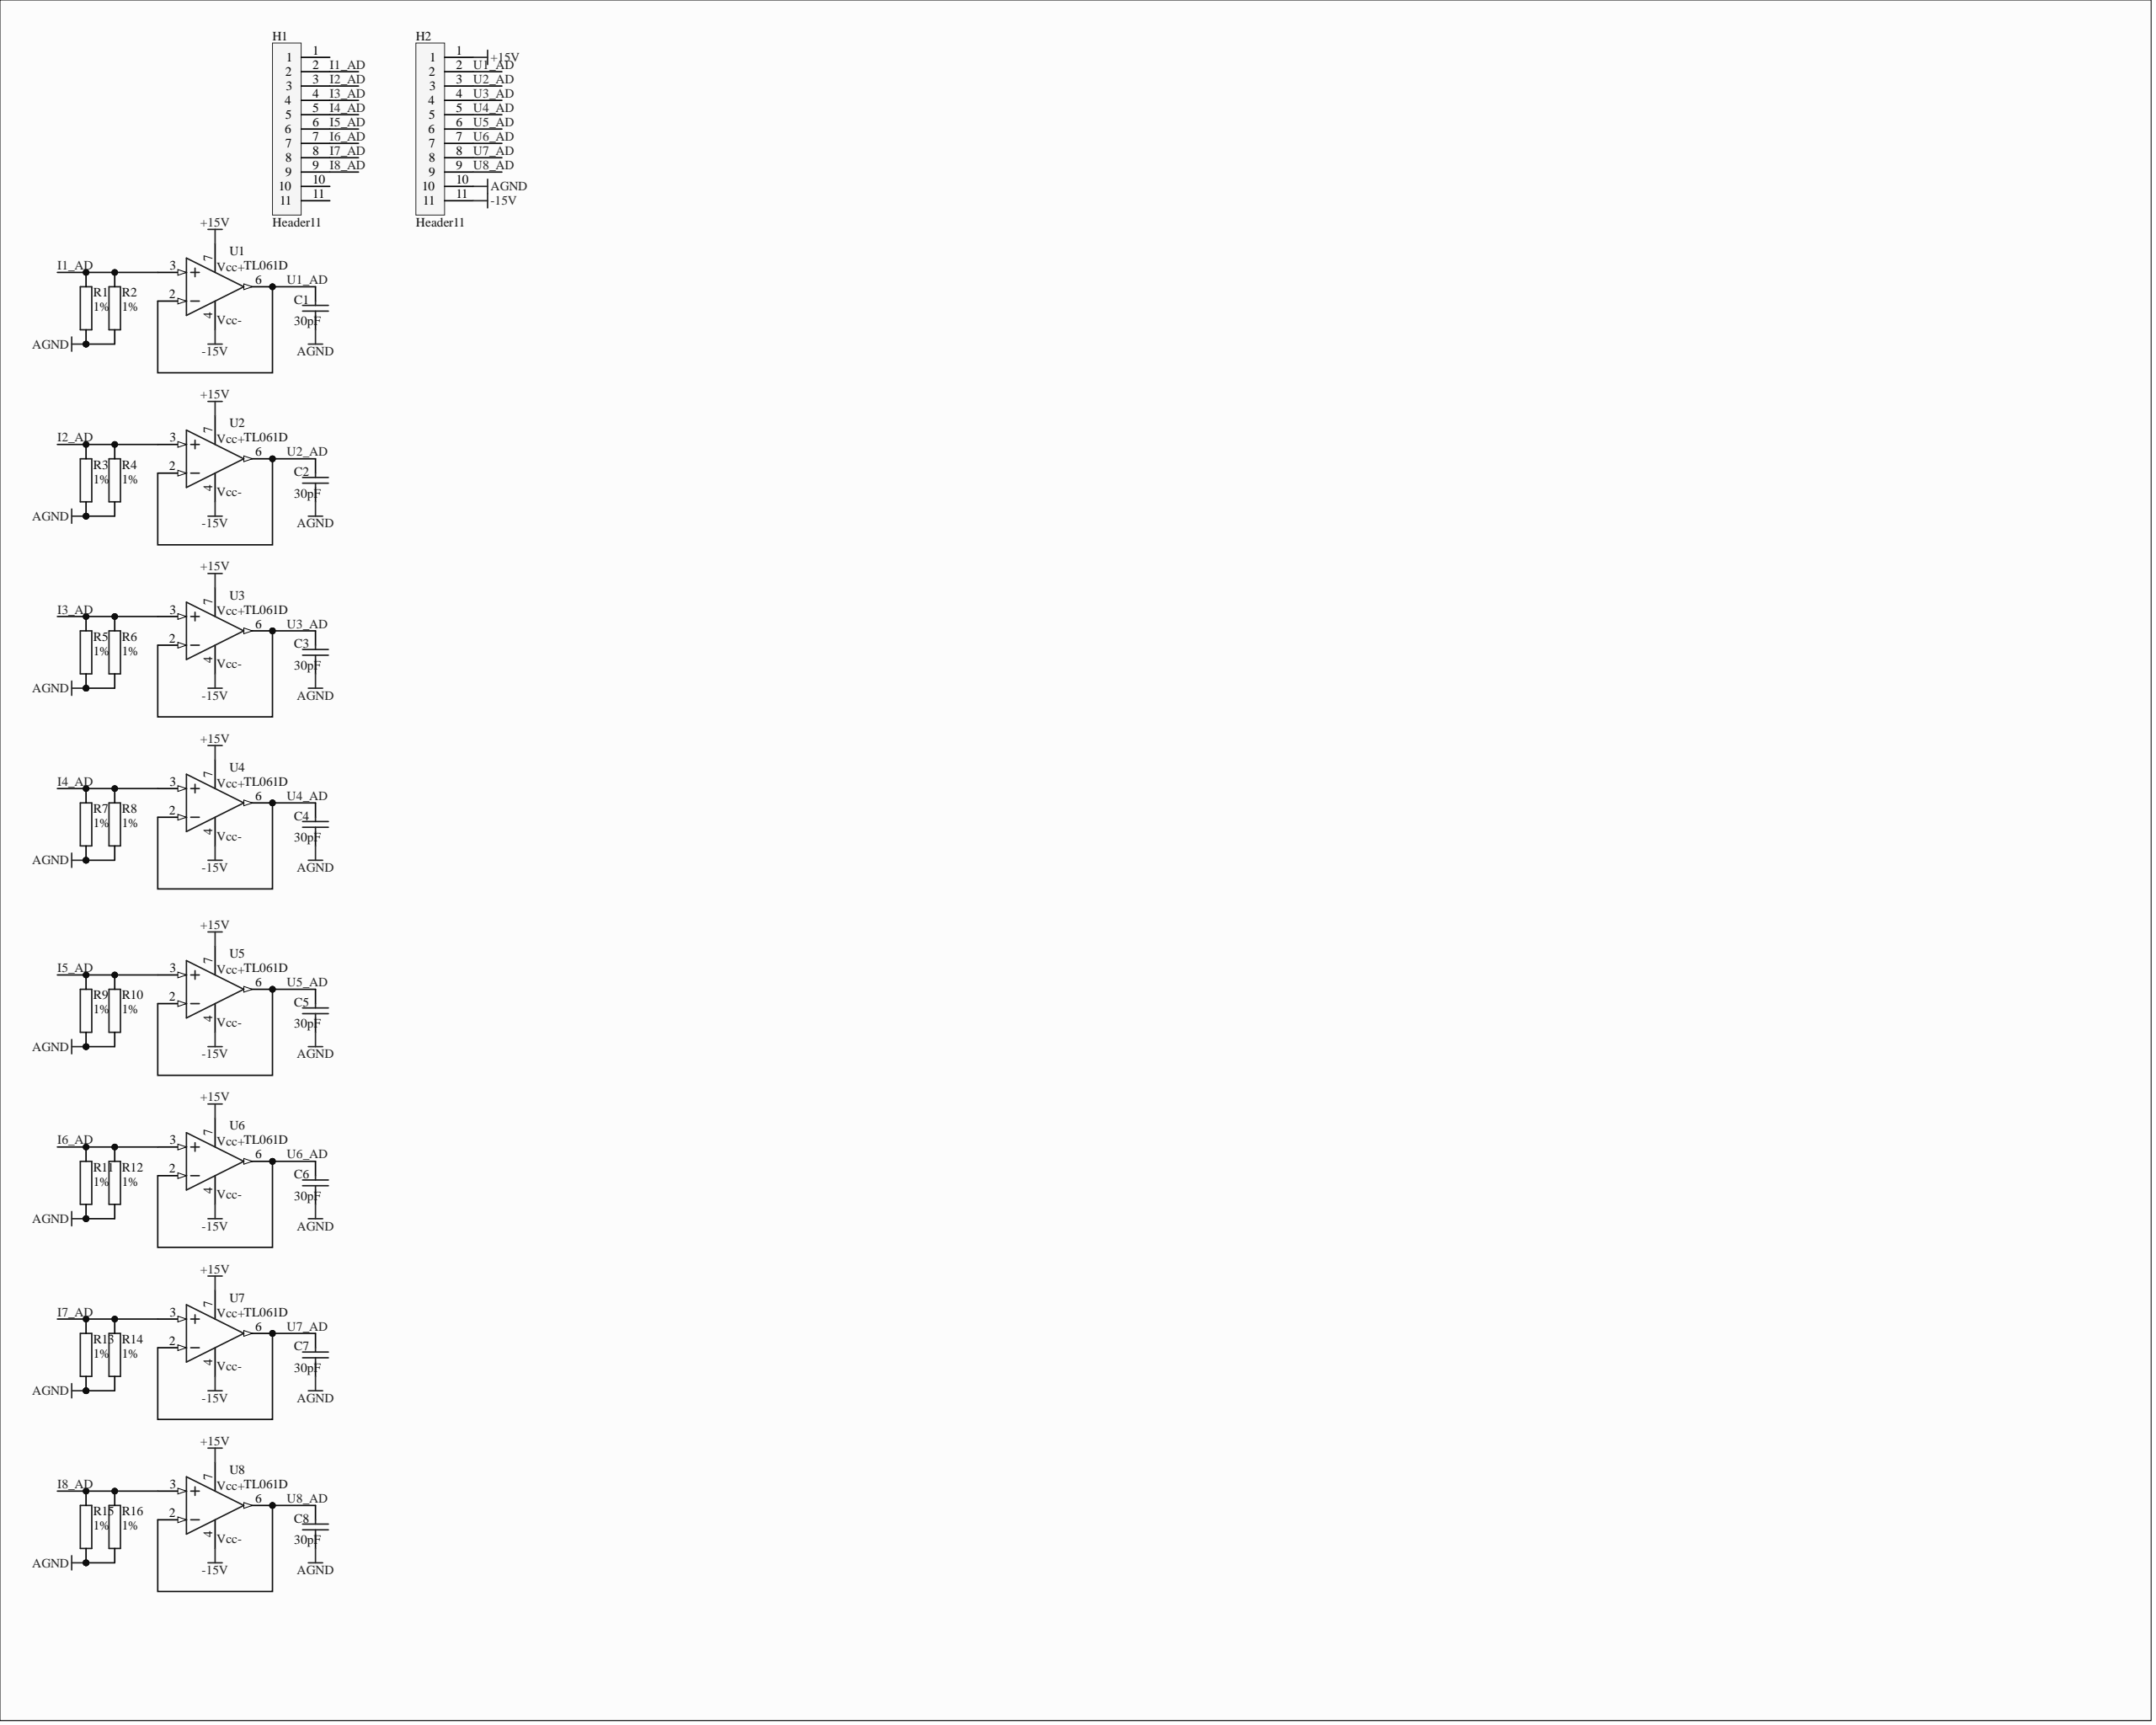Circuit board | Altium Designer | 34 parts | 19 nets
Bill of materials:
Comment,Description,Designator,Footprint,LibRef,Quantity
"30pF","Capacitor","C1, C2, C3, C4, C5, C6, C7, C8","0603","CAP","8"
"Header11","Header11","H1, H2","PinHeader11_1.27mm","Header11","2"
"1%","","R1, R2, R3, R4, R5, R6, R7, R8, R9, R10, R11, R12, R13, R14, R15, R16","1206","ProE260.TMP_300K_25","16"
"TL061D","TL061D","U1, U2, U3, U4, U5, U6, U7, U8","TL061_SOIC8","TL061D","8"
Netlist (Protel format):
[
C1
0603
30pF



]
[
C2
0603
30pF



]
[
C3
0603
30pF



]
[
C4
0603
30pF



]
[
C5
0603
30pF



]
[
C6
0603
30pF



]
[
C7
0603
30pF



]
[
C8
0603
30pF



]
[
H1
PinHeader11_1.27mm
Header11



]
[
H2
PinHeader11_1.27mm
Header11



]
[
R1
1206
1%



]
[
R2
1206
1%



]
[
R3
1206
1%



]
[
R4
1206
1%



]
[
R5
1206
1%



]
[
R6
1206
1%



]
[
R7
1206
1%



]
[
R8
1206
1%



]
[
R9
1206
1%



]
[
R10
1206
1%



]
[
R11
1206
1%



]
[
R12
1206
1%



]
[
R13
1206
1%



]
[
R14
1206
1%



]
[
R15
1206
1%



]
[
R16
1206
1%



]
[
U1
TL061_SOIC8
TL061D



]
[
U2
TL061_SOIC8
TL061D



]
[
U3
TL061_SOIC8
TL061D



]
[
U4
TL061_SOIC8
TL061D



]
[
U5
TL061_SOIC8
TL061D



]
[
U6
TL061_SOIC8
TL061D



]
[
U7
TL061_SOIC8
TL061D



]
[
U8
TL061_SOIC8
TL061D



]
(
U8_AD
C8-2
H2-9
U8-2
U8-6
)
(
U7_AD
C7-2
H2-8
U7-2
U7-6
)
(
U6_AD
C6-2
H2-7
U6-2
U6-6
)
(
U5_AD
C5-2
H2-6
U5-2
U5-6
)
(
U4_AD
C4-2
H2-5
U4-2
U4-6
)
(
U3_AD
C3-2
H2-4
U3-2
U3-6
)
(
U2_AD
C2-2
H2-3
U2-2
U2-6
)
(
U1_AD
C1-2
H2-2
U1-2
U1-6
)
(
I8_AD
H1-9
R15-1
R16-1
U8-3
)
(
I7_AD
H1-8
R13-1
R14-1
U7-3
)
(
I6_AD
H1-7
R11-1
R12-1
U6-3
)
(
I5_AD
H1-6
R9-1
R10-1
U5-3
)
(
I4_AD
H1-5
R7-1
R8-1
U4-3
)
(
I3_AD
H1-4
R5-1
R6-1
U3-3
)
(
I2_AD
H1-3
R3-1
R4-1
U2-3
)
(
I1_AD
H1-2
R1-1
R2-1
U1-3
)
(
AGND
C1-1
C2-1
C3-1
C4-1
C5-1
C6-1
C7-1
C8-1
H2-10
R1-2
R2-2
R3-2
R4-2
R5-2
R6-2
R7-2
R8-2
R9-2
R10-2
R11-2
R12-2
R13-2
R14-2
R15-2
R16-2
)
(
-15V
H2-11
U1-4
U2-4
U3-4
U4-4
U5-4
U6-4
U7-4
U8-4
)
(
+15V
H2-1
U1-7
U2-7
U3-7
U4-7
U5-7
U6-7
U7-7
U8-7
)